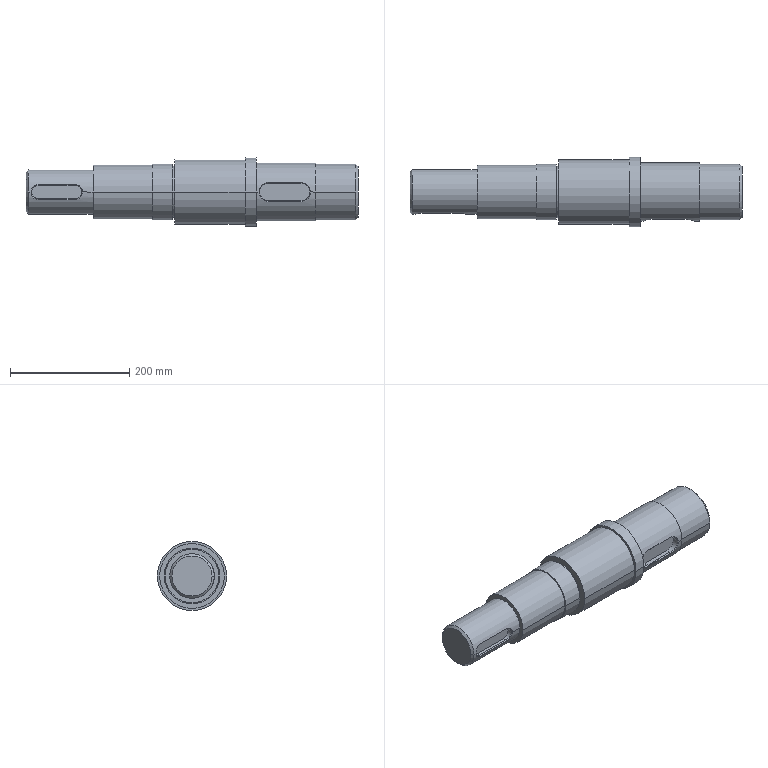Part | SolidWorks | features ICE 4, Chamfer 1, Revolution 1, Scale 1 | 1 solid | 47 faces | box 556.875 x 116.25 x 116.25 mm | volume 3869573 mm3 | cylinder 20 | plane 19 | cone 4 | spline 4 | commonest cylinder face diameters 93.75 x4 22.5 x2 30 x2 75 x2 86.25 x2 90 x2